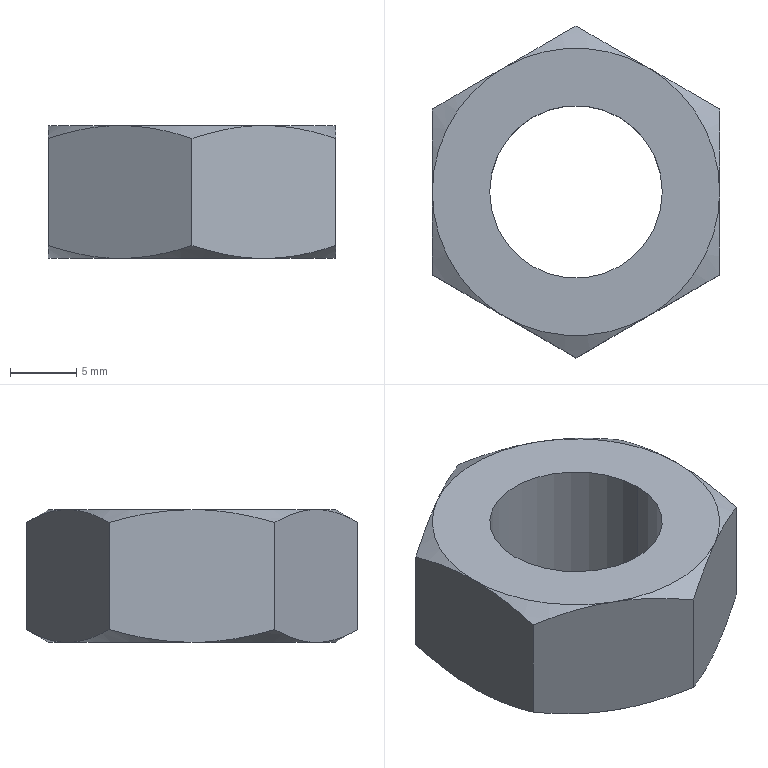Part | SolidWorks | features ICE 2, Extrusion 1, MirrorPattern 1 | 1 solid | 22 faces | box 21.651 x 25 x 10 mm | volume 2710 mm3 | cone 12 | plane 8 | cylinder 2 | commonest cylinder face diameters 13 x2
STEP:
#1=CARTESIAN_POINT('',(6.5,0.,5.));
#2=VERTEX_POINT('',#1);
#3=CARTESIAN_POINT('',(-6.5,0.,5.));
#4=VERTEX_POINT('',#3);
#5=CARTESIAN_POINT('',(0.,0.,5.));
#6=DIRECTION('',(0.,0.,-1.));
#7=DIRECTION('',(-1.,0.,0.));
#8=AXIS2_PLACEMENT_3D('',#5,#6,#7);
#9=CIRCLE('',#8,6.5);
#10=EDGE_CURVE('',#2,#4,#9,.T.);
#11=ORIENTED_EDGE('',*,*,#10,.F.);
#12=CARTESIAN_POINT('',(6.5,0.,-5.));
#13=VERTEX_POINT('',#12);
#14=CARTESIAN_POINT('',(6.5,0.,5.));
#15=DIRECTION('',(0.,0.,-1.));
#16=VECTOR('',#15,1000.);
#17=LINE('',#14,#16);
#18=EDGE_CURVE('',#2,#13,#17,.T.);
#19=ORIENTED_EDGE('',*,*,#18,.T.);
#20=CARTESIAN_POINT('',(-6.5,0.,-5.));
#21=VERTEX_POINT('',#20);
#22=CARTESIAN_POINT('',(0.,0.,-5.));
#23=DIRECTION('',(0.,0.,-1.));
#24=DIRECTION('',(-1.,0.,0.));
#25=AXIS2_PLACEMENT_3D('',#22,#23,#24);
#26=CIRCLE('',#25,6.5);
#27=EDGE_CURVE('',#13,#21,#26,.T.);
#28=ORIENTED_EDGE('',*,*,#27,.T.);
#29=CARTESIAN_POINT('',(-6.5,0.,5.));
#30=DIRECTION('',(0.,0.,-1.));
#31=VECTOR('',#30,1000.);
#32=LINE('',#29,#31);
#33=EDGE_CURVE('',#4,#21,#32,.T.);
#34=ORIENTED_EDGE('',*,*,#33,.F.);
#35=EDGE_LOOP('',(#11,#19,#28,#34));
#36=FACE_OUTER_BOUND('',#35,.T.);
#37=CARTESIAN_POINT('',(0.,0.,5.));
#38=DIRECTION('',(0.,0.,-1.));
#39=DIRECTION('',(-1.,0.,0.));
#40=AXIS2_PLACEMENT_3D('',#37,#38,#39);
#41=CYLINDRICAL_SURFACE('',#40,6.5);
#42=ADVANCED_FACE('',(#36),#41,.F.);
#43=CARTESIAN_POINT('',(10.825,6.25,4.033));
#44=VERTEX_POINT('',#43);
#45=CARTESIAN_POINT('',(10.825,6.25,-4.033));
#46=VERTEX_POINT('',#45);
#47=CARTESIAN_POINT('',(10.825,6.25,5.));
#48=DIRECTION('',(0.,0.,-1.));
#49=VECTOR('',#48,1000.);
#50=LINE('',#47,#49);
#51=EDGE_CURVE('',#44,#46,#50,.T.);
#52=ORIENTED_EDGE('',*,*,#51,.T.);
#53=CARTESIAN_POINT('',(5.413,9.375,-5.));
#54=VERTEX_POINT('',#53);
#55=CARTESIAN_POINT('',(10.825,6.25,-4.033));
#56=CARTESIAN_POINT('',(9.94,6.761,-4.328));
#57=CARTESIAN_POINT('',(9.048,7.276,-4.571));
#58=CARTESIAN_POINT('',(7.246,8.317,-4.908));
#59=CARTESIAN_POINT('',(6.335,8.843,-5.));
#60=CARTESIAN_POINT('',(5.413,9.375,-5.));
#61=B_SPLINE_CURVE_WITH_KNOTS('',3,(#55,#56,#57,#58,#59,#60),.UNSPECIFIED.,.F.,.F.,(4,2,4),(0.000000238,0.003162,0.006324),.UNSPECIFIED.);
#62=EDGE_CURVE('',#46,#54,#61,.T.);
#63=ORIENTED_EDGE('',*,*,#62,.T.);
#64=CARTESIAN_POINT('',(0.,12.5,-4.033));
#65=VERTEX_POINT('',#64);
#66=CARTESIAN_POINT('',(5.413,9.375,-5.));
#67=CARTESIAN_POINT('',(4.953,9.64,-5.));
#68=CARTESIAN_POINT('',(4.492,9.907,-4.977));
#69=CARTESIAN_POINT('',(3.579,10.434,-4.889));
#70=CARTESIAN_POINT('',(3.126,10.695,-4.823));
#71=CARTESIAN_POINT('',(1.774,11.476,-4.571));
#72=CARTESIAN_POINT('',(0.8832,11.99,-4.328));
#73=CARTESIAN_POINT('',(0.,12.5,-4.033));
#74=B_SPLINE_CURVE_WITH_KNOTS('',3,(#66,#67,#68,#69,#70,#71,#72,#73),.UNSPECIFIED.,.F.,.F.,(4,2,2,4),(0.006324,0.007899,0.009474,0.01262),.UNSPECIFIED.);
#75=EDGE_CURVE('',#54,#65,#74,.T.);
#76=ORIENTED_EDGE('',*,*,#75,.T.);
#77=CARTESIAN_POINT('',(0.,12.5,4.033));
#78=VERTEX_POINT('',#77);
#79=CARTESIAN_POINT('',(0.,12.5,5.));
#80=DIRECTION('',(0.,0.,-1.));
#81=VECTOR('',#80,1000.);
#82=LINE('',#79,#81);
#83=EDGE_CURVE('',#78,#65,#82,.T.);
#84=ORIENTED_EDGE('',*,*,#83,.F.);
#85=CARTESIAN_POINT('',(5.413,9.375,5.));
#86=VERTEX_POINT('',#85);
#87=CARTESIAN_POINT('',(5.413,9.375,5.));
#88=CARTESIAN_POINT('',(4.953,9.64,5.));
#89=CARTESIAN_POINT('',(4.492,9.907,4.977));
#90=CARTESIAN_POINT('',(3.579,10.434,4.889));
#91=CARTESIAN_POINT('',(3.126,10.695,4.823));
#92=CARTESIAN_POINT('',(1.774,11.476,4.571));
#93=CARTESIAN_POINT('',(0.8832,11.99,4.328));
#94=CARTESIAN_POINT('',(0.,12.5,4.033));
#95=B_SPLINE_CURVE_WITH_KNOTS('',3,(#87,#88,#89,#90,#91,#92,#93,#94),.UNSPECIFIED.,.F.,.F.,(4,2,2,4),(0.006324,0.007899,0.009474,0.01262),.UNSPECIFIED.);
#96=EDGE_CURVE('',#86,#78,#95,.T.);
#97=ORIENTED_EDGE('',*,*,#96,.F.);
#98=CARTESIAN_POINT('',(10.825,6.25,4.033));
#99=CARTESIAN_POINT('',(9.94,6.761,4.328));
#100=CARTESIAN_POINT('',(9.048,7.276,4.571));
#101=CARTESIAN_POINT('',(7.246,8.317,4.908));
#102=CARTESIAN_POINT('',(6.335,8.843,5.));
#103=CARTESIAN_POINT('',(5.413,9.375,5.));
#104=B_SPLINE_CURVE_WITH_KNOTS('',3,(#98,#99,#100,#101,#102,#103),.UNSPECIFIED.,.F.,.F.,(4,2,4),(0.000000238,0.003162,0.006324),.UNSPECIFIED.);
#105=EDGE_CURVE('',#44,#86,#104,.T.);
#106=ORIENTED_EDGE('',*,*,#105,.F.);
#107=EDGE_LOOP('',(#52,#63,#76,#84,#97,#106));
#108=FACE_OUTER_BOUND('',#107,.T.);
#109=CARTESIAN_POINT('',(10.825,6.25,5.));
#110=DIRECTION('',(-0.5,-0.866,0.));
#111=DIRECTION('',(0.866,-0.5,0.));
#112=AXIS2_PLACEMENT_3D('',#109,#110,#111);
#113=PLANE('',#112);
#114=ADVANCED_FACE('',(#108),#113,.F.);
#115=ORIENTED_EDGE('',*,*,#83,.T.);
#116=CARTESIAN_POINT('',(-5.413,9.375,-5.));
#117=VERTEX_POINT('',#116);
#118=CARTESIAN_POINT('',(0.,12.5,-4.033));
#119=CARTESIAN_POINT('',(-0.8854,11.989,-4.328));
#120=CARTESIAN_POINT('',(-1.777,11.474,-4.571));
#121=CARTESIAN_POINT('',(-3.58,10.433,-4.908));
#122=CARTESIAN_POINT('',(-4.491,9.907,-5.));
#123=CARTESIAN_POINT('',(-5.413,9.375,-5.));
#124=B_SPLINE_CURVE_WITH_KNOTS('',3,(#118,#119,#120,#121,#122,#123),.UNSPECIFIED.,.F.,.F.,(4,2,4),(0.000000238,0.003162,0.006324),.UNSPECIFIED.);
#125=EDGE_CURVE('',#65,#117,#124,.T.);
#126=ORIENTED_EDGE('',*,*,#125,.T.);
#127=CARTESIAN_POINT('',(-10.825,6.25,-4.033));
#128=VERTEX_POINT('',#127);
#129=CARTESIAN_POINT('',(-5.413,9.375,-5.));
#130=CARTESIAN_POINT('',(-5.872,9.11,-5.));
#131=CARTESIAN_POINT('',(-6.333,8.843,-4.977));
#132=CARTESIAN_POINT('',(-7.246,8.316,-4.889));
#133=CARTESIAN_POINT('',(-7.7,8.055,-4.823));
#134=CARTESIAN_POINT('',(-9.051,7.274,-4.571));
#135=CARTESIAN_POINT('',(-9.942,6.76,-4.328));
#136=CARTESIAN_POINT('',(-10.825,6.25,-4.033));
#137=B_SPLINE_CURVE_WITH_KNOTS('',3,(#129,#130,#131,#132,#133,#134,#135,#136),.UNSPECIFIED.,.F.,.F.,(4,2,2,4),(0.006324,0.007899,0.009474,0.01262),.UNSPECIFIED.);
#138=EDGE_CURVE('',#117,#128,#137,.T.);
#139=ORIENTED_EDGE('',*,*,#138,.T.);
#140=CARTESIAN_POINT('',(-10.825,6.25,4.033));
#141=VERTEX_POINT('',#140);
#142=CARTESIAN_POINT('',(-10.825,6.25,5.));
#143=DIRECTION('',(0.,0.,-1.));
#144=VECTOR('',#143,1000.);
#145=LINE('',#142,#144);
#146=EDGE_CURVE('',#141,#128,#145,.T.);
#147=ORIENTED_EDGE('',*,*,#146,.F.);
#148=CARTESIAN_POINT('',(-5.413,9.375,5.));
#149=VERTEX_POINT('',#148);
#150=CARTESIAN_POINT('',(-5.413,9.375,5.));
#151=CARTESIAN_POINT('',(-5.872,9.11,5.));
#152=CARTESIAN_POINT('',(-6.333,8.843,4.977));
#153=CARTESIAN_POINT('',(-7.246,8.316,4.889));
#154=CARTESIAN_POINT('',(-7.7,8.055,4.823));
#155=CARTESIAN_POINT('',(-9.051,7.274,4.571));
#156=CARTESIAN_POINT('',(-9.942,6.76,4.328));
#157=CARTESIAN_POINT('',(-10.825,6.25,4.033));
#158=B_SPLINE_CURVE_WITH_KNOTS('',3,(#150,#151,#152,#153,#154,#155,#156,#157),.UNSPECIFIED.,.F.,.F.,(4,2,2,4),(0.006324,0.007899,0.009474,0.01262),.UNSPECIFIED.);
#159=EDGE_CURVE('',#149,#141,#158,.T.);
#160=ORIENTED_EDGE('',*,*,#159,.F.);
#161=CARTESIAN_POINT('',(0.,12.5,4.033));
#162=CARTESIAN_POINT('',(-0.8854,11.989,4.328));
#163=CARTESIAN_POINT('',(-1.777,11.474,4.571));
#164=CARTESIAN_POINT('',(-3.58,10.433,4.908));
#165=CARTESIAN_POINT('',(-4.491,9.907,5.));
#166=CARTESIAN_POINT('',(-5.413,9.375,5.));
#167=B_SPLINE_CURVE_WITH_KNOTS('',3,(#161,#162,#163,#164,#165,#166),.UNSPECIFIED.,.F.,.F.,(4,2,4),(0.000000238,0.003162,0.006324),.UNSPECIFIED.);
#168=EDGE_CURVE('',#78,#149,#167,.T.);
#169=ORIENTED_EDGE('',*,*,#168,.F.);
#170=EDGE_LOOP('',(#115,#126,#139,#147,#160,#169));
#171=FACE_OUTER_BOUND('',#170,.T.);
#172=CARTESIAN_POINT('',(0.,12.5,5.));
#173=DIRECTION('',(0.5,-0.866,0.));
#174=DIRECTION('',(0.866,0.5,0.));
#175=AXIS2_PLACEMENT_3D('',#172,#173,#174);
#176=PLANE('',#175);
#177=ADVANCED_FACE('',(#171),#176,.F.);
#178=ORIENTED_EDGE('',*,*,#146,.T.);
#179=CARTESIAN_POINT('',(-10.825,0.,-5.));
#180=VERTEX_POINT('',#179);
#181=CARTESIAN_POINT('',(-10.825,6.25,-4.033));
#182=CARTESIAN_POINT('',(-10.825,5.237,-4.326));
#183=CARTESIAN_POINT('',(-10.825,4.213,-4.568));
#184=CARTESIAN_POINT('',(-10.825,2.65,-4.822));
#185=CARTESIAN_POINT('',(-10.825,2.124,-4.888));
#186=CARTESIAN_POINT('',(-10.825,1.063,-4.977));
#187=CARTESIAN_POINT('',(-10.825,0.5287,-5.));
#188=CARTESIAN_POINT('',(-10.825,0.,-5.));
#189=B_SPLINE_CURVE_WITH_KNOTS('',3,(#181,#182,#183,#184,#185,#186,#187,#188),.UNSPECIFIED.,.F.,.F.,(4,2,2,4),(0.01712,0.0203,0.02188,0.02347),.UNSPECIFIED.);
#190=EDGE_CURVE('',#128,#180,#189,.T.);
#191=ORIENTED_EDGE('',*,*,#190,.T.);
#192=CARTESIAN_POINT('',(-10.825,-6.25,-4.033));
#193=VERTEX_POINT('',#192);
#194=CARTESIAN_POINT('',(-10.825,0.,-5.));
#195=CARTESIAN_POINT('',(-10.825,-1.065,-5.));
#196=CARTESIAN_POINT('',(-10.825,-2.116,-4.908));
#197=CARTESIAN_POINT('',(-10.825,-4.198,-4.571));
#198=CARTESIAN_POINT('',(-10.825,-5.228,-4.328));
#199=CARTESIAN_POINT('',(-10.825,-6.25,-4.033));
#200=B_SPLINE_CURVE_WITH_KNOTS('',3,(#194,#195,#196,#197,#198,#199),.UNSPECIFIED.,.F.,.F.,(4,2,4),(0.02347,0.02667,0.02986),.UNSPECIFIED.);
#201=EDGE_CURVE('',#180,#193,#200,.T.);
#202=ORIENTED_EDGE('',*,*,#201,.T.);
#203=CARTESIAN_POINT('',(-10.825,-6.25,4.033));
#204=VERTEX_POINT('',#203);
#205=CARTESIAN_POINT('',(-10.825,-6.25,5.));
#206=DIRECTION('',(0.,0.,-1.));
#207=VECTOR('',#206,1000.);
#208=LINE('',#205,#207);
#209=EDGE_CURVE('',#204,#193,#208,.T.);
#210=ORIENTED_EDGE('',*,*,#209,.F.);
#211=CARTESIAN_POINT('',(-10.825,0.,5.));
#212=VERTEX_POINT('',#211);
#213=CARTESIAN_POINT('',(-10.825,0.,5.));
#214=CARTESIAN_POINT('',(-10.825,-1.065,5.));
#215=CARTESIAN_POINT('',(-10.825,-2.116,4.908));
#216=CARTESIAN_POINT('',(-10.825,-4.198,4.571));
#217=CARTESIAN_POINT('',(-10.825,-5.228,4.328));
#218=CARTESIAN_POINT('',(-10.825,-6.25,4.033));
#219=B_SPLINE_CURVE_WITH_KNOTS('',3,(#213,#214,#215,#216,#217,#218),.UNSPECIFIED.,.F.,.F.,(4,2,4),(0.02347,0.02667,0.02986),.UNSPECIFIED.);
#220=EDGE_CURVE('',#212,#204,#219,.T.);
#221=ORIENTED_EDGE('',*,*,#220,.F.);
#222=CARTESIAN_POINT('',(-10.825,6.25,4.033));
#223=CARTESIAN_POINT('',(-10.825,5.237,4.326));
#224=CARTESIAN_POINT('',(-10.825,4.213,4.568));
#225=CARTESIAN_POINT('',(-10.825,2.65,4.822));
#226=CARTESIAN_POINT('',(-10.825,2.124,4.888));
#227=CARTESIAN_POINT('',(-10.825,1.063,4.977));
#228=CARTESIAN_POINT('',(-10.825,0.5287,5.));
#229=CARTESIAN_POINT('',(-10.825,0.,5.));
#230=B_SPLINE_CURVE_WITH_KNOTS('',3,(#222,#223,#224,#225,#226,#227,#228,#229),.UNSPECIFIED.,.F.,.F.,(4,2,2,4),(0.01712,0.0203,0.02188,0.02347),.UNSPECIFIED.);
#231=EDGE_CURVE('',#141,#212,#230,.T.);
#232=ORIENTED_EDGE('',*,*,#231,.F.);
#233=EDGE_LOOP('',(#178,#191,#202,#210,#221,#232));
#234=FACE_OUTER_BOUND('',#233,.T.);
#235=CARTESIAN_POINT('',(-10.825,6.25,5.));
#236=DIRECTION('',(1.,0.,0.));
#237=DIRECTION('',(0.,1.,0.));
#238=AXIS2_PLACEMENT_3D('',#235,#236,#237);
#239=PLANE('',#238);
#240=ADVANCED_FACE('',(#234),#239,.F.);
#241=ORIENTED_EDGE('',*,*,#209,.T.);
#242=CARTESIAN_POINT('',(-5.413,-9.375,-5.));
#243=VERTEX_POINT('',#242);
#244=CARTESIAN_POINT('',(-10.825,-6.25,-4.033));
#245=CARTESIAN_POINT('',(-9.94,-6.761,-4.328));
#246=CARTESIAN_POINT('',(-9.048,-7.276,-4.571));
#247=CARTESIAN_POINT('',(-7.246,-8.317,-4.908));
#248=CARTESIAN_POINT('',(-6.335,-8.843,-5.));
#249=CARTESIAN_POINT('',(-5.413,-9.375,-5.));
#250=B_SPLINE_CURVE_WITH_KNOTS('',3,(#244,#245,#246,#247,#248,#249),.UNSPECIFIED.,.F.,.F.,(4,2,4),(0.000000238,0.003162,0.006324),.UNSPECIFIED.);
#251=EDGE_CURVE('',#193,#243,#250,.T.);
#252=ORIENTED_EDGE('',*,*,#251,.T.);
#253=CARTESIAN_POINT('',(0.,-12.5,-4.033));
#254=VERTEX_POINT('',#253);
#255=CARTESIAN_POINT('',(-5.413,-9.375,-5.));
#256=CARTESIAN_POINT('',(-4.953,-9.64,-5.));
#257=CARTESIAN_POINT('',(-4.492,-9.907,-4.977));
#258=CARTESIAN_POINT('',(-3.579,-10.434,-4.889));
#259=CARTESIAN_POINT('',(-3.126,-10.695,-4.823));
#260=CARTESIAN_POINT('',(-1.774,-11.476,-4.571));
#261=CARTESIAN_POINT('',(-0.8832,-11.99,-4.328));
#262=CARTESIAN_POINT('',(0.,-12.5,-4.033));
#263=B_SPLINE_CURVE_WITH_KNOTS('',3,(#255,#256,#257,#258,#259,#260,#261,#262),.UNSPECIFIED.,.F.,.F.,(4,2,2,4),(0.006324,0.007899,0.009474,0.01262),.UNSPECIFIED.);
#264=EDGE_CURVE('',#243,#254,#263,.T.);
#265=ORIENTED_EDGE('',*,*,#264,.T.);
#266=CARTESIAN_POINT('',(0.,-12.5,4.033));
#267=VERTEX_POINT('',#266);
#268=CARTESIAN_POINT('',(0.,-12.5,5.));
#269=DIRECTION('',(0.,0.,-1.));
#270=VECTOR('',#269,1000.);
#271=LINE('',#268,#270);
#272=EDGE_CURVE('',#267,#254,#271,.T.);
#273=ORIENTED_EDGE('',*,*,#272,.F.);
#274=CARTESIAN_POINT('',(-5.413,-9.375,5.));
#275=VERTEX_POINT('',#274);
#276=CARTESIAN_POINT('',(-5.413,-9.375,5.));
#277=CARTESIAN_POINT('',(-4.953,-9.64,5.));
#278=CARTESIAN_POINT('',(-4.492,-9.907,4.977));
#279=CARTESIAN_POINT('',(-3.579,-10.434,4.889));
#280=CARTESIAN_POINT('',(-3.126,-10.695,4.823));
#281=CARTESIAN_POINT('',(-1.774,-11.476,4.571));
#282=CARTESIAN_POINT('',(-0.8832,-11.99,4.328));
#283=CARTESIAN_POINT('',(0.,-12.5,4.033));
#284=B_SPLINE_CURVE_WITH_KNOTS('',3,(#276,#277,#278,#279,#280,#281,#282,#283),.UNSPECIFIED.,.F.,.F.,(4,2,2,4),(0.006324,0.007899,0.009474,0.01262),.UNSPECIFIED.);
#285=EDGE_CURVE('',#275,#267,#284,.T.);
#286=ORIENTED_EDGE('',*,*,#285,.F.);
#287=CARTESIAN_POINT('',(-10.825,-6.25,4.033));
#288=CARTESIAN_POINT('',(-9.94,-6.761,4.328));
#289=CARTESIAN_POINT('',(-9.048,-7.276,4.571));
#290=CARTESIAN_POINT('',(-7.246,-8.317,4.908));
#291=CARTESIAN_POINT('',(-6.335,-8.843,5.));
#292=CARTESIAN_POINT('',(-5.413,-9.375,5.));
#293=B_SPLINE_CURVE_WITH_KNOTS('',3,(#287,#288,#289,#290,#291,#292),.UNSPECIFIED.,.F.,.F.,(4,2,4),(0.000000238,0.003162,0.006324),.UNSPECIFIED.);
#294=EDGE_CURVE('',#204,#275,#293,.T.);
#295=ORIENTED_EDGE('',*,*,#294,.F.);
#296=EDGE_LOOP('',(#241,#252,#265,#273,#286,#295));
#297=FACE_OUTER_BOUND('',#296,.T.);
#298=CARTESIAN_POINT('',(-10.825,-6.25,5.));
#299=DIRECTION('',(0.5,0.866,0.));
#300=DIRECTION('',(-0.866,0.5,0.));
#301=AXIS2_PLACEMENT_3D('',#298,#299,#300);
#302=PLANE('',#301);
#303=ADVANCED_FACE('',(#297),#302,.F.);
#304=ORIENTED_EDGE('',*,*,#272,.T.);
#305=CARTESIAN_POINT('',(5.413,-9.375,-5.));
#306=VERTEX_POINT('',#305);
#307=CARTESIAN_POINT('',(0.,-12.5,-4.033));
#308=CARTESIAN_POINT('',(0.8854,-11.989,-4.328));
#309=CARTESIAN_POINT('',(1.777,-11.474,-4.571));
#310=CARTESIAN_POINT('',(3.58,-10.433,-4.908));
#311=CARTESIAN_POINT('',(4.491,-9.907,-5.));
#312=CARTESIAN_POINT('',(5.413,-9.375,-5.));
#313=B_SPLINE_CURVE_WITH_KNOTS('',3,(#307,#308,#309,#310,#311,#312),.UNSPECIFIED.,.F.,.F.,(4,2,4),(0.000000238,0.003162,0.006324),.UNSPECIFIED.);
#314=EDGE_CURVE('',#254,#306,#313,.T.);
#315=ORIENTED_EDGE('',*,*,#314,.T.);
#316=CARTESIAN_POINT('',(10.825,-6.25,-4.033));
#317=VERTEX_POINT('',#316);
#318=CARTESIAN_POINT('',(5.413,-9.375,-5.));
#319=CARTESIAN_POINT('',(5.872,-9.11,-5.));
#320=CARTESIAN_POINT('',(6.333,-8.843,-4.977));
#321=CARTESIAN_POINT('',(7.246,-8.316,-4.889));
#322=CARTESIAN_POINT('',(7.7,-8.055,-4.823));
#323=CARTESIAN_POINT('',(9.051,-7.274,-4.571));
#324=CARTESIAN_POINT('',(9.942,-6.76,-4.328));
#325=CARTESIAN_POINT('',(10.825,-6.25,-4.033));
#326=B_SPLINE_CURVE_WITH_KNOTS('',3,(#318,#319,#320,#321,#322,#323,#324,#325),.UNSPECIFIED.,.F.,.F.,(4,2,2,4),(0.006324,0.007899,0.009474,0.01262),.UNSPECIFIED.);
#327=EDGE_CURVE('',#306,#317,#326,.T.);
#328=ORIENTED_EDGE('',*,*,#327,.T.);
#329=CARTESIAN_POINT('',(10.825,-6.25,4.033));
#330=VERTEX_POINT('',#329);
#331=CARTESIAN_POINT('',(10.825,-6.25,5.));
#332=DIRECTION('',(0.,0.,-1.));
#333=VECTOR('',#332,1000.);
#334=LINE('',#331,#333);
#335=EDGE_CURVE('',#330,#317,#334,.T.);
#336=ORIENTED_EDGE('',*,*,#335,.F.);
#337=CARTESIAN_POINT('',(5.413,-9.375,5.));
#338=VERTEX_POINT('',#337);
#339=CARTESIAN_POINT('',(5.413,-9.375,5.));
#340=CARTESIAN_POINT('',(5.872,-9.11,5.));
#341=CARTESIAN_POINT('',(6.333,-8.843,4.977));
#342=CARTESIAN_POINT('',(7.246,-8.316,4.889));
#343=CARTESIAN_POINT('',(7.7,-8.055,4.823));
#344=CARTESIAN_POINT('',(9.051,-7.274,4.571));
#345=CARTESIAN_POINT('',(9.942,-6.76,4.328));
#346=CARTESIAN_POINT('',(10.825,-6.25,4.033));
#347=B_SPLINE_CURVE_WITH_KNOTS('',3,(#339,#340,#341,#342,#343,#344,#345,#346),.UNSPECIFIED.,.F.,.F.,(4,2,2,4),(0.006324,0.007899,0.009474,0.01262),.UNSPECIFIED.);
#348=EDGE_CURVE('',#338,#330,#347,.T.);
#349=ORIENTED_EDGE('',*,*,#348,.F.);
#350=CARTESIAN_POINT('',(0.,-12.5,4.033));
#351=CARTESIAN_POINT('',(0.8854,-11.989,4.328));
#352=CARTESIAN_POINT('',(1.777,-11.474,4.571));
#353=CARTESIAN_POINT('',(3.58,-10.433,4.908));
#354=CARTESIAN_POINT('',(4.491,-9.907,5.));
#355=CARTESIAN_POINT('',(5.413,-9.375,5.));
#356=B_SPLINE_CURVE_WITH_KNOTS('',3,(#350,#351,#352,#353,#354,#355),.UNSPECIFIED.,.F.,.F.,(4,2,4),(0.000000238,0.003162,0.006324),.UNSPECIFIED.);
#357=EDGE_CURVE('',#267,#338,#356,.T.);
#358=ORIENTED_EDGE('',*,*,#357,.F.);
#359=EDGE_LOOP('',(#304,#315,#328,#336,#349,#358));
#360=FACE_OUTER_BOUND('',#359,.T.);
#361=CARTESIAN_POINT('',(0.,-12.5,5.));
#362=DIRECTION('',(-0.5,0.866,0.));
#363=DIRECTION('',(-0.866,-0.5,0.));
#364=AXIS2_PLACEMENT_3D('',#361,#362,#363);
#365=PLANE('',#364);
#366=ADVANCED_FACE('',(#360),#365,.F.);
#367=ORIENTED_EDGE('',*,*,#335,.T.);
#368=CARTESIAN_POINT('',(10.825,0.,-5.));
#369=VERTEX_POINT('',#368);
#370=CARTESIAN_POINT('',(10.825,-6.25,-4.033));
#371=CARTESIAN_POINT('',(10.825,-5.237,-4.326));
#372=CARTESIAN_POINT('',(10.825,-4.213,-4.568));
#373=CARTESIAN_POINT('',(10.825,-2.65,-4.822));
#374=CARTESIAN_POINT('',(10.825,-2.124,-4.888));
#375=CARTESIAN_POINT('',(10.825,-1.063,-4.977));
#376=CARTESIAN_POINT('',(10.825,-0.5287,-5.));
#377=CARTESIAN_POINT('',(10.825,0.,-5.));
#378=B_SPLINE_CURVE_WITH_KNOTS('',3,(#370,#371,#372,#373,#374,#375,#376,#377),.UNSPECIFIED.,.F.,.F.,(4,2,2,4),(0.01712,0.0203,0.02188,0.02347),.UNSPECIFIED.);
#379=EDGE_CURVE('',#317,#369,#378,.T.);
#380=ORIENTED_EDGE('',*,*,#379,.T.);
#381=CARTESIAN_POINT('',(10.825,0.,-5.));
#382=CARTESIAN_POINT('',(10.825,1.065,-5.));
#383=CARTESIAN_POINT('',(10.825,2.116,-4.908));
#384=CARTESIAN_POINT('',(10.825,4.198,-4.571));
#385=CARTESIAN_POINT('',(10.825,5.228,-4.328));
#386=CARTESIAN_POINT('',(10.825,6.25,-4.033));
#387=B_SPLINE_CURVE_WITH_KNOTS('',3,(#381,#382,#383,#384,#385,#386),.UNSPECIFIED.,.F.,.F.,(4,2,4),(0.02347,0.02667,0.02986),.UNSPECIFIED.);
#388=EDGE_CURVE('',#369,#46,#387,.T.);
#389=ORIENTED_EDGE('',*,*,#388,.T.);
#390=ORIENTED_EDGE('',*,*,#51,.F.);
#391=CARTESIAN_POINT('',(10.825,0.,5.));
#392=VERTEX_POINT('',#391);
#393=CARTESIAN_POINT('',(10.825,0.,5.));
#394=CARTESIAN_POINT('',(10.825,1.065,5.));
#395=CARTESIAN_POINT('',(10.825,2.116,4.908));
#396=CARTESIAN_POINT('',(10.825,4.198,4.571));
#397=CARTESIAN_POINT('',(10.825,5.228,4.328));
#398=CARTESIAN_POINT('',(10.825,6.25,4.033));
#399=B_SPLINE_CURVE_WITH_KNOTS('',3,(#393,#394,#395,#396,#397,#398),.UNSPECIFIED.,.F.,.F.,(4,2,4),(0.02347,0.02667,0.02986),.UNSPECIFIED.);
#400=EDGE_CURVE('',#392,#44,#399,.T.);
#401=ORIENTED_EDGE('',*,*,#400,.F.);
#402=CARTESIAN_POINT('',(10.825,-6.25,4.033));
#403=CARTESIAN_POINT('',(10.825,-5.237,4.326));
#404=CARTESIAN_POINT('',(10.825,-4.213,4.568));
#405=CARTESIAN_POINT('',(10.825,-2.65,4.822));
#406=CARTESIAN_POINT('',(10.825,-2.124,4.888));
#407=CARTESIAN_POINT('',(10.825,-1.063,4.977));
#408=CARTESIAN_POINT('',(10.825,-0.5287,5.));
#409=CARTESIAN_POINT('',(10.825,0.,5.));
#410=B_SPLINE_CURVE_WITH_KNOTS('',3,(#402,#403,#404,#405,#406,#407,#408,#409),.UNSPECIFIED.,.F.,.F.,(4,2,2,4),(0.01712,0.0203,0.02188,0.02347),.UNSPECIFIED.);
#411=EDGE_CURVE('',#330,#392,#410,.T.);
#412=ORIENTED_EDGE('',*,*,#411,.F.);
#413=EDGE_LOOP('',(#367,#380,#389,#390,#401,#412));
#414=FACE_OUTER_BOUND('',#413,.T.);
#415=CARTESIAN_POINT('',(10.825,-6.25,5.));
#416=DIRECTION('',(-1.,0.,0.));
#417=DIRECTION('',(0.,0.,1.));
#418=AXIS2_PLACEMENT_3D('',#415,#416,#417);
#419=PLANE('',#418);
#420=ADVANCED_FACE('',(#414),#419,.F.);
#421=ORIENTED_EDGE('',*,*,#348,.T.);
#422=ORIENTED_EDGE('',*,*,#411,.T.);
#423=CARTESIAN_POINT('',(0.,0.,5.));
#424=DIRECTION('',(0.,0.,1.));
#425=DIRECTION('',(1.,0.,0.));
#426=AXIS2_PLACEMENT_3D('',#423,#424,#425);
#427=CIRCLE('',#426,10.825);
#428=EDGE_CURVE('',#338,#392,#427,.T.);
#429=ORIENTED_EDGE('',*,*,#428,.F.);
#430=EDGE_LOOP('',(#421,#422,#429));
#431=FACE_OUTER_BOUND('',#430,.T.);
#432=CARTESIAN_POINT('',(0.,0.,5.));
#433=DIRECTION('',(0.,0.,-1.));
#434=DIRECTION('',(1.,0.,0.));
#435=AXIS2_PLACEMENT_3D('',#432,#433,#434);
#436=CONICAL_SURFACE('',#435,10.825,1.047);
#437=ADVANCED_FACE('',(#431),#436,.T.);
#438=ORIENTED_EDGE('',*,*,#285,.T.);
#439=ORIENTED_EDGE('',*,*,#357,.T.);
#440=CARTESIAN_POINT('',(0.,0.,5.));
#441=DIRECTION('',(0.,0.,1.));
#442=DIRECTION('',(1.,0.,0.));
#443=AXIS2_PLACEMENT_3D('',#440,#441,#442);
#444=CIRCLE('',#443,10.825);
#445=EDGE_CURVE('',#275,#338,#444,.T.);
#446=ORIENTED_EDGE('',*,*,#445,.F.);
#447=EDGE_LOOP('',(#438,#439,#446));
#448=FACE_OUTER_BOUND('',#447,.T.);
#449=CARTESIAN_POINT('',(0.,0.,5.));
#450=DIRECTION('',(0.,0.,-1.));
#451=DIRECTION('',(1.,0.,0.));
#452=AXIS2_PLACEMENT_3D('',#449,#450,#451);
#453=CONICAL_SURFACE('',#452,10.825,1.047);
#454=ADVANCED_FACE('',(#448),#453,.T.);
#455=ORIENTED_EDGE('',*,*,#220,.T.);
#456=ORIENTED_EDGE('',*,*,#294,.T.);
#457=CARTESIAN_POINT('',(0.,0.,5.));
#458=DIRECTION('',(0.,0.,1.));
#459=DIRECTION('',(1.,0.,0.));
#460=AXIS2_PLACEMENT_3D('',#457,#458,#459);
#461=CIRCLE('',#460,10.825);
#462=EDGE_CURVE('',#212,#275,#461,.T.);
#463=ORIENTED_EDGE('',*,*,#462,.F.);
#464=EDGE_LOOP('',(#455,#456,#463));
#465=FACE_OUTER_BOUND('',#464,.T.);
#466=CARTESIAN_POINT('',(0.,0.,5.));
#467=DIRECTION('',(0.,0.,-1.));
#468=DIRECTION('',(1.,0.,0.));
#469=AXIS2_PLACEMENT_3D('',#466,#467,#468);
#470=CONICAL_SURFACE('',#469,10.825,1.047);
#471=ADVANCED_FACE('',(#465),#470,.T.);
#472=ORIENTED_EDGE('',*,*,#159,.T.);
#473=ORIENTED_EDGE('',*,*,#231,.T.);
#474=CARTESIAN_POINT('',(0.,0.,5.));
#475=DIRECTION('',(0.,0.,1.));
#476=DIRECTION('',(1.,0.,0.));
#477=AXIS2_PLACEMENT_3D('',#474,#475,#476);
#478=CIRCLE('',#477,10.825);
#479=EDGE_CURVE('',#149,#212,#478,.T.);
#480=ORIENTED_EDGE('',*,*,#479,.F.);
#481=EDGE_LOOP('',(#472,#473,#480));
#482=FACE_OUTER_BOUND('',#481,.T.);
#483=CARTESIAN_POINT('',(0.,0.,5.));
#484=DIRECTION('',(0.,0.,-1.));
#485=DIRECTION('',(1.,0.,0.));
#486=AXIS2_PLACEMENT_3D('',#483,#484,#485);
#487=CONICAL_SURFACE('',#486,10.825,1.047);
#488=ADVANCED_FACE('',(#482),#487,.T.);
#489=ORIENTED_EDGE('',*,*,#96,.T.);
#490=ORIENTED_EDGE('',*,*,#168,.T.);
#491=CARTESIAN_POINT('',(0.,0.,5.));
#492=DIRECTION('',(0.,0.,1.));
#493=DIRECTION('',(1.,0.,0.));
#494=AXIS2_PLACEMENT_3D('',#491,#492,#493);
#495=CIRCLE('',#494,10.825);
#496=EDGE_CURVE('',#86,#149,#495,.T.);
#497=ORIENTED_EDGE('',*,*,#496,.F.);
#498=EDGE_LOOP('',(#489,#490,#497));
#499=FACE_OUTER_BOUND('',#498,.T.);
#500=CARTESIAN_POINT('',(0.,0.,5.));
#501=DIRECTION('',(0.,0.,-1.));
#502=DIRECTION('',(1.,0.,0.));
#503=AXIS2_PLACEMENT_3D('',#500,#501,#502);
#504=CONICAL_SURFACE('',#503,10.825,1.047);
#505=ADVANCED_FACE('',(#499),#504,.T.);
#506=ORIENTED_EDGE('',*,*,#105,.T.);
#507=CARTESIAN_POINT('',(0.,0.,5.));
#508=DIRECTION('',(0.,0.,1.));
#509=DIRECTION('',(1.,0.,0.));
#510=AXIS2_PLACEMENT_3D('',#507,#508,#509);
#511=CIRCLE('',#510,10.825);
#512=EDGE_CURVE('',#392,#86,#511,.T.);
#513=ORIENTED_EDGE('',*,*,#512,.F.);
#514=ORIENTED_EDGE('',*,*,#400,.T.);
#515=EDGE_LOOP('',(#506,#513,#514));
#516=FACE_OUTER_BOUND('',#515,.T.);
#517=CARTESIAN_POINT('',(0.,0.,5.));
#518=DIRECTION('',(0.,0.,-1.));
#519=DIRECTION('',(1.,0.,0.));
#520=AXIS2_PLACEMENT_3D('',#517,#518,#519);
#521=CONICAL_SURFACE('',#520,10.825,1.047);
#522=ADVANCED_FACE('',(#516),#521,.T.);
#523=CARTESIAN_POINT('',(0.,0.,5.));
#524=DIRECTION('',(0.,0.,-1.));
#525=DIRECTION('',(-1.,0.,0.));
#526=AXIS2_PLACEMENT_3D('',#523,#524,#525);
#527=CIRCLE('',#526,6.5);
#528=EDGE_CURVE('',#4,#2,#527,.T.);
#529=ORIENTED_EDGE('',*,*,#528,.T.);
#530=ORIENTED_EDGE('',*,*,#10,.T.);
#531=EDGE_LOOP('',(#529,#530));
#532=FACE_BOUND('',#531,.T.);
#533=ORIENTED_EDGE('',*,*,#428,.T.);
#534=ORIENTED_EDGE('',*,*,#512,.T.);
#535=ORIENTED_EDGE('',*,*,#496,.T.);
#536=ORIENTED_EDGE('',*,*,#479,.T.);
#537=ORIENTED_EDGE('',*,*,#462,.T.);
#538=ORIENTED_EDGE('',*,*,#445,.T.);
#539=EDGE_LOOP('',(#533,#534,#535,#536,#537,#538));
#540=FACE_OUTER_BOUND('',#539,.T.);
#541=CARTESIAN_POINT('',(0.,0.,5.));
#542=DIRECTION('',(0.,0.,1.));
#543=DIRECTION('',(1.,0.,0.));
#544=AXIS2_PLACEMENT_3D('',#541,#542,#543);
#545=PLANE('',#544);
#546=ADVANCED_FACE('',(#532,#540),#545,.T.);
#547=ORIENTED_EDGE('',*,*,#388,.F.);
#548=CARTESIAN_POINT('',(0.,0.,-5.));
#549=DIRECTION('',(0.,0.,1.));
#550=DIRECTION('',(1.,0.,0.));
#551=AXIS2_PLACEMENT_3D('',#548,#549,#550);
#552=CIRCLE('',#551,10.825);
#553=EDGE_CURVE('',#369,#54,#552,.T.);
#554=ORIENTED_EDGE('',*,*,#553,.T.);
#555=ORIENTED_EDGE('',*,*,#62,.F.);
#556=EDGE_LOOP('',(#547,#554,#555));
#557=FACE_OUTER_BOUND('',#556,.T.);
#558=CARTESIAN_POINT('',(0.,0.,-5.));
#559=DIRECTION('',(0.,0.,1.));
#560=DIRECTION('',(1.,0.,0.));
#561=AXIS2_PLACEMENT_3D('',#558,#559,#560);
#562=CONICAL_SURFACE('',#561,10.825,1.047);
#563=ADVANCED_FACE('',(#557),#562,.T.);
#564=CARTESIAN_POINT('',(0.,0.,-5.));
#565=DIRECTION('',(0.,0.,-1.));
#566=DIRECTION('',(1.,0.,0.));
#567=AXIS2_PLACEMENT_3D('',#564,#565,#566);
#568=CIRCLE('',#567,10.825);
#569=EDGE_CURVE('',#117,#54,#568,.T.);
#570=ORIENTED_EDGE('',*,*,#569,.F.);
#571=ORIENTED_EDGE('',*,*,#125,.F.);
#572=ORIENTED_EDGE('',*,*,#75,.F.);
#573=EDGE_LOOP('',(#570,#571,#572));
#574=FACE_OUTER_BOUND('',#573,.T.);
#575=CARTESIAN_POINT('',(0.,0.,-5.));
#576=DIRECTION('',(0.,0.,1.));
#577=DIRECTION('',(1.,0.,0.));
#578=AXIS2_PLACEMENT_3D('',#575,#576,#577);
#579=CONICAL_SURFACE('',#578,10.825,1.047);
#580=ADVANCED_FACE('',(#574),#579,.T.);
#581=CARTESIAN_POINT('',(0.,0.,-5.));
#582=DIRECTION('',(0.,0.,-1.));
#583=DIRECTION('',(1.,0.,0.));
#584=AXIS2_PLACEMENT_3D('',#581,#582,#583);
#585=CIRCLE('',#584,10.825);
#586=EDGE_CURVE('',#180,#117,#585,.T.);
#587=ORIENTED_EDGE('',*,*,#586,.F.);
#588=ORIENTED_EDGE('',*,*,#190,.F.);
#589=ORIENTED_EDGE('',*,*,#138,.F.);
#590=EDGE_LOOP('',(#587,#588,#589));
#591=FACE_OUTER_BOUND('',#590,.T.);
#592=CARTESIAN_POINT('',(0.,0.,-5.));
#593=DIRECTION('',(0.,0.,1.));
#594=DIRECTION('',(1.,0.,0.));
#595=AXIS2_PLACEMENT_3D('',#592,#593,#594);
#596=CONICAL_SURFACE('',#595,10.825,1.047);
#597=ADVANCED_FACE('',(#591),#596,.T.);
#598=CARTESIAN_POINT('',(0.,0.,-5.));
#599=DIRECTION('',(0.,0.,-1.));
#600=DIRECTION('',(1.,0.,0.));
#601=AXIS2_PLACEMENT_3D('',#598,#599,#600);
#602=CIRCLE('',#601,10.825);
#603=EDGE_CURVE('',#243,#180,#602,.T.);
#604=ORIENTED_EDGE('',*,*,#603,.F.);
#605=ORIENTED_EDGE('',*,*,#251,.F.);
#606=ORIENTED_EDGE('',*,*,#201,.F.);
#607=EDGE_LOOP('',(#604,#605,#606));
#608=FACE_OUTER_BOUND('',#607,.T.);
#609=CARTESIAN_POINT('',(0.,0.,-5.));
#610=DIRECTION('',(0.,0.,1.));
#611=DIRECTION('',(1.,0.,0.));
#612=AXIS2_PLACEMENT_3D('',#609,#610,#611);
#613=CONICAL_SURFACE('',#612,10.825,1.047);
#614=ADVANCED_FACE('',(#608),#613,.T.);
#615=CARTESIAN_POINT('',(0.,0.,-5.));
#616=DIRECTION('',(0.,0.,-1.));
#617=DIRECTION('',(1.,0.,0.));
#618=AXIS2_PLACEMENT_3D('',#615,#616,#617);
#619=CIRCLE('',#618,10.825);
#620=EDGE_CURVE('',#306,#243,#619,.T.);
#621=ORIENTED_EDGE('',*,*,#620,.F.);
#622=ORIENTED_EDGE('',*,*,#314,.F.);
#623=ORIENTED_EDGE('',*,*,#264,.F.);
#624=EDGE_LOOP('',(#621,#622,#623));
#625=FACE_OUTER_BOUND('',#624,.T.);
#626=CARTESIAN_POINT('',(0.,0.,-5.));
#627=DIRECTION('',(0.,0.,1.));
#628=DIRECTION('',(1.,0.,0.));
#629=AXIS2_PLACEMENT_3D('',#626,#627,#628);
#630=CONICAL_SURFACE('',#629,10.825,1.047);
#631=ADVANCED_FACE('',(#625),#630,.T.);
#632=CARTESIAN_POINT('',(0.,0.,-5.));
#633=DIRECTION('',(0.,0.,-1.));
#634=DIRECTION('',(1.,0.,0.));
#635=AXIS2_PLACEMENT_3D('',#632,#633,#634);
#636=CIRCLE('',#635,10.825);
#637=EDGE_CURVE('',#369,#306,#636,.T.);
#638=ORIENTED_EDGE('',*,*,#637,.F.);
#639=ORIENTED_EDGE('',*,*,#379,.F.);
#640=ORIENTED_EDGE('',*,*,#327,.F.);
#641=EDGE_LOOP('',(#638,#639,#640));
#642=FACE_OUTER_BOUND('',#641,.T.);
#643=CARTESIAN_POINT('',(0.,0.,-5.));
#644=DIRECTION('',(0.,0.,1.));
#645=DIRECTION('',(1.,0.,0.));
#646=AXIS2_PLACEMENT_3D('',#643,#644,#645);
#647=CONICAL_SURFACE('',#646,10.825,1.047);
#648=ADVANCED_FACE('',(#642),#647,.T.);
#649=CARTESIAN_POINT('',(0.,0.,-5.));
#650=DIRECTION('',(0.,0.,-1.));
#651=DIRECTION('',(-1.,0.,0.));
#652=AXIS2_PLACEMENT_3D('',#649,#650,#651);
#653=CIRCLE('',#652,6.5);
#654=EDGE_CURVE('',#21,#13,#653,.T.);
#655=ORIENTED_EDGE('',*,*,#654,.F.);
#656=ORIENTED_EDGE('',*,*,#27,.F.);
#657=EDGE_LOOP('',(#655,#656));
#658=FACE_BOUND('',#657,.T.);
#659=ORIENTED_EDGE('',*,*,#553,.F.);
#660=ORIENTED_EDGE('',*,*,#637,.T.);
#661=ORIENTED_EDGE('',*,*,#620,.T.);
#662=ORIENTED_EDGE('',*,*,#603,.T.);
#663=ORIENTED_EDGE('',*,*,#586,.T.);
#664=ORIENTED_EDGE('',*,*,#569,.T.);
#665=EDGE_LOOP('',(#659,#660,#661,#662,#663,#664));
#666=FACE_OUTER_BOUND('',#665,.T.);
#667=CARTESIAN_POINT('',(0.,0.,-5.));
#668=DIRECTION('',(0.,0.,1.));
#669=DIRECTION('',(1.,0.,0.));
#670=AXIS2_PLACEMENT_3D('',#667,#668,#669);
#671=PLANE('',#670);
#672=ADVANCED_FACE('',(#658,#666),#671,.F.);
#673=ORIENTED_EDGE('',*,*,#18,.F.);
#674=ORIENTED_EDGE('',*,*,#528,.F.);
#675=ORIENTED_EDGE('',*,*,#33,.T.);
#676=ORIENTED_EDGE('',*,*,#654,.T.);
#677=EDGE_LOOP('',(#673,#674,#675,#676));
#678=FACE_OUTER_BOUND('',#677,.T.);
#679=CARTESIAN_POINT('',(0.,0.,5.));
#680=DIRECTION('',(0.,0.,-1.));
#681=DIRECTION('',(-1.,0.,0.));
#682=AXIS2_PLACEMENT_3D('',#679,#680,#681);
#683=CYLINDRICAL_SURFACE('',#682,6.5);
#684=ADVANCED_FACE('',(#678),#683,.F.);
#685=CLOSED_SHELL('',(#42,#114,#177,#240,#303,#366,#420,#437,#454,#471,#488,#505,#522,#546,#563,#580,#597,#614,#631,#648,#672,#684));
#686=MANIFOLD_SOLID_BREP('',#685);
#687=CARTESIAN_POINT('',(0.,0.,0.));
#688=DIRECTION('',(0.,0.,1.));
#689=DIRECTION('',(1.,0.,0.));
#690=AXIS2_PLACEMENT_3D('',#687,#688,#689);
#691=(LENGTH_UNIT()NAMED_UNIT(*)SI_UNIT(.MILLI.,.METRE.));
#692=UNCERTAINTY_MEASURE_WITH_UNIT(LENGTH_MEASURE(0.00001),#691,'','');
#693=(NAMED_UNIT(*)PLANE_ANGLE_UNIT()SI_UNIT($,.RADIAN.));
#694=(NAMED_UNIT(*)SI_UNIT($,.STERADIAN.)SOLID_ANGLE_UNIT());
#695=(GEOMETRIC_REPRESENTATION_CONTEXT(3)GLOBAL_UNCERTAINTY_ASSIGNED_CONTEXT((#692))GLOBAL_UNIT_ASSIGNED_CONTEXT((#691,#693,#694))REPRESENTATION_CONTEXT('',''));
#696=ADVANCED_BREP_SHAPE_REPRESENTATION('',(#686,#690),#695);